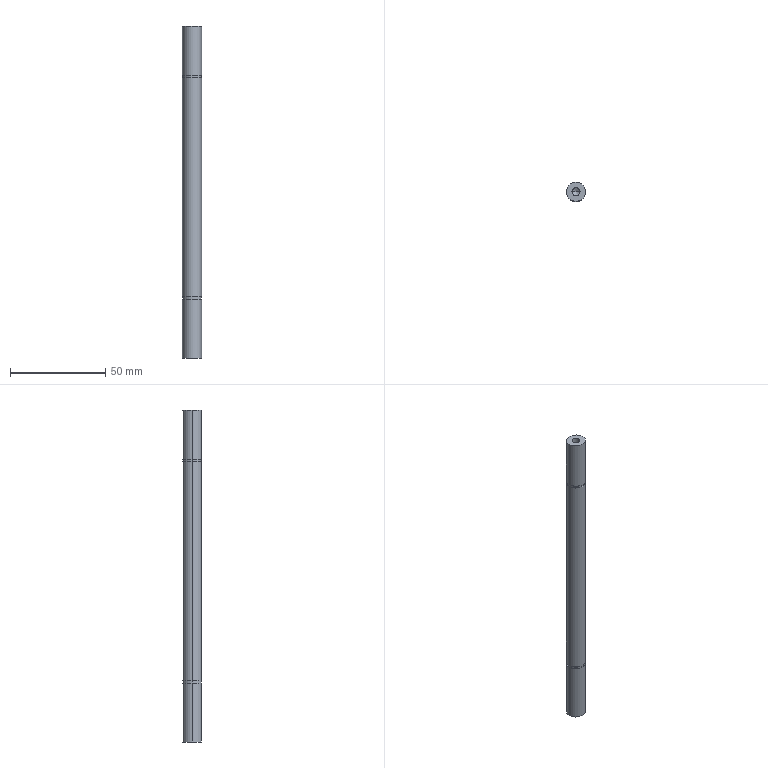Part | SolidWorks | features HoleWzd 2, Extrusion 1, RevCut 1 | 1 solid | 24 faces | box 10 x 10 x 174 mm | volume 13253 mm3 | cylinder 14 | plane 6 | cone 4 | commonest cylinder face diameters 10 x6 4.2 x4 9.6 x4
STEP:
#1=CARTESIAN_POINT('',(5.,0.,-56.1));
#2=VERTEX_POINT('',#1);
#3=CARTESIAN_POINT('',(-5.,0.,-56.1));
#4=VERTEX_POINT('',#3);
#5=CARTESIAN_POINT('',(0.,0.,-56.1));
#6=DIRECTION('',(0.,0.,1.));
#7=DIRECTION('',(1.,0.,0.));
#8=AXIS2_PLACEMENT_3D('',#5,#6,#7);
#9=CIRCLE('',#8,5.);
#10=EDGE_CURVE('',#2,#4,#9,.T.);
#11=ORIENTED_EDGE('',*,*,#10,.F.);
#12=CARTESIAN_POINT('',(5.,0.,-87.));
#13=VERTEX_POINT('',#12);
#14=CARTESIAN_POINT('',(5.,0.,87.));
#15=DIRECTION('',(0.,0.,-1.));
#16=VECTOR('',#15,1000.);
#17=LINE('',#14,#16);
#18=EDGE_CURVE('',#2,#13,#17,.T.);
#19=ORIENTED_EDGE('',*,*,#18,.T.);
#20=CARTESIAN_POINT('',(-5.,0.,-87.));
#21=VERTEX_POINT('',#20);
#22=CARTESIAN_POINT('',(0.,0.,-87.));
#23=DIRECTION('',(0.,0.,1.));
#24=DIRECTION('',(1.,0.,0.));
#25=AXIS2_PLACEMENT_3D('',#22,#23,#24);
#26=CIRCLE('',#25,5.);
#27=EDGE_CURVE('',#13,#21,#26,.T.);
#28=ORIENTED_EDGE('',*,*,#27,.T.);
#29=CARTESIAN_POINT('',(-5.,0.,87.));
#30=DIRECTION('',(0.,0.,-1.));
#31=VECTOR('',#30,1000.);
#32=LINE('',#29,#31);
#33=EDGE_CURVE('',#4,#21,#32,.T.);
#34=ORIENTED_EDGE('',*,*,#33,.F.);
#35=EDGE_LOOP('',(#11,#19,#28,#34));
#36=FACE_OUTER_BOUND('',#35,.T.);
#37=CARTESIAN_POINT('',(0.,0.,87.));
#38=DIRECTION('',(0.,0.,-1.));
#39=DIRECTION('',(-1.,0.,0.));
#40=AXIS2_PLACEMENT_3D('',#37,#38,#39);
#41=CYLINDRICAL_SURFACE('',#40,5.);
#42=ADVANCED_FACE('',(#36),#41,.T.);
#43=CARTESIAN_POINT('',(2.1,0.,-73.));
#44=VERTEX_POINT('',#43);
#45=CARTESIAN_POINT('',(-2.1,0.,-73.));
#46=VERTEX_POINT('',#45);
#47=CARTESIAN_POINT('',(0.,0.,-73.));
#48=DIRECTION('',(0.,0.,-1.));
#49=DIRECTION('',(-1.,0.,0.));
#50=AXIS2_PLACEMENT_3D('',#47,#48,#49);
#51=CIRCLE('',#50,2.1);
#52=EDGE_CURVE('',#44,#46,#51,.T.);
#53=ORIENTED_EDGE('',*,*,#52,.F.);
#54=CARTESIAN_POINT('',(2.1,0.,-87.));
#55=VERTEX_POINT('',#54);
#56=CARTESIAN_POINT('',(2.1,0.,-87.));
#57=DIRECTION('',(0.,0.,-1.));
#58=VECTOR('',#57,1000.);
#59=LINE('',#56,#58);
#60=EDGE_CURVE('',#44,#55,#59,.T.);
#61=ORIENTED_EDGE('',*,*,#60,.T.);
#62=CARTESIAN_POINT('',(-2.1,0.,-87.));
#63=VERTEX_POINT('',#62);
#64=CARTESIAN_POINT('',(0.,0.,-87.));
#65=DIRECTION('',(0.,0.,-1.));
#66=DIRECTION('',(-1.,0.,0.));
#67=AXIS2_PLACEMENT_3D('',#64,#65,#66);
#68=CIRCLE('',#67,2.1);
#69=EDGE_CURVE('',#55,#63,#68,.T.);
#70=ORIENTED_EDGE('',*,*,#69,.T.);
#71=CARTESIAN_POINT('',(-2.1,0.,-87.));
#72=DIRECTION('',(0.,0.,-1.));
#73=VECTOR('',#72,1000.);
#74=LINE('',#71,#73);
#75=EDGE_CURVE('',#46,#63,#74,.T.);
#76=ORIENTED_EDGE('',*,*,#75,.F.);
#77=EDGE_LOOP('',(#53,#61,#70,#76));
#78=FACE_OUTER_BOUND('',#77,.T.);
#79=CARTESIAN_POINT('',(0.,0.,-87.));
#80=DIRECTION('',(0.,0.,-1.));
#81=DIRECTION('',(-1.,0.,0.));
#82=AXIS2_PLACEMENT_3D('',#79,#80,#81);
#83=CYLINDRICAL_SURFACE('',#82,2.1);
#84=ADVANCED_FACE('',(#78),#83,.F.);
#85=CARTESIAN_POINT('',(0.,0.,-71.738));
#86=VERTEX_POINT('',#85);
#87=CARTESIAN_POINT('',(-2.1,0.,-73.));
#88=DIRECTION('',(-0.8572,0.,-0.515));
#89=VECTOR('',#88,1000.);
#90=LINE('',#87,#89);
#91=EDGE_CURVE('',#86,#46,#90,.T.);
#92=ORIENTED_EDGE('',*,*,#91,.F.);
#93=CARTESIAN_POINT('',(2.1,0.,-73.));
#94=DIRECTION('',(0.8572,0.,-0.515));
#95=VECTOR('',#94,1000.);
#96=LINE('',#93,#95);
#97=EDGE_CURVE('',#86,#44,#96,.T.);
#98=ORIENTED_EDGE('',*,*,#97,.T.);
#99=ORIENTED_EDGE('',*,*,#52,.T.);
#100=EDGE_LOOP('',(#92,#98,#99));
#101=FACE_OUTER_BOUND('',#100,.T.);
#102=CARTESIAN_POINT('',(0.,0.,-73.));
#103=DIRECTION('',(0.,0.,-1.));
#104=DIRECTION('',(-1.,0.,0.));
#105=AXIS2_PLACEMENT_3D('',#102,#103,#104);
#106=CONICAL_SURFACE('',#105,2.1,1.03);
#107=ADVANCED_FACE('',(#101),#106,.F.);
#108=CARTESIAN_POINT('',(4.8,0.,-56.1));
#109=VERTEX_POINT('',#108);
#110=CARTESIAN_POINT('',(-4.8,0.,-56.1));
#111=VERTEX_POINT('',#110);
#112=CARTESIAN_POINT('',(0.,0.,-56.1));
#113=DIRECTION('',(0.,0.,1.));
#114=DIRECTION('',(1.,0.,0.));
#115=AXIS2_PLACEMENT_3D('',#112,#113,#114);
#116=CIRCLE('',#115,4.8);
#117=EDGE_CURVE('',#109,#111,#116,.T.);
#118=ORIENTED_EDGE('',*,*,#117,.T.);
#119=CARTESIAN_POINT('',(-4.8,0.,-55.));
#120=VERTEX_POINT('',#119);
#121=CARTESIAN_POINT('',(-4.8,0.,87.));
#122=DIRECTION('',(0.,0.,1.));
#123=VECTOR('',#122,1000.);
#124=LINE('',#121,#123);
#125=EDGE_CURVE('',#111,#120,#124,.T.);
#126=ORIENTED_EDGE('',*,*,#125,.T.);
#127=CARTESIAN_POINT('',(4.8,0.,-55.));
#128=VERTEX_POINT('',#127);
#129=CARTESIAN_POINT('',(0.,0.,-55.));
#130=DIRECTION('',(0.,0.,1.));
#131=DIRECTION('',(1.,0.,0.));
#132=AXIS2_PLACEMENT_3D('',#129,#130,#131);
#133=CIRCLE('',#132,4.8);
#134=EDGE_CURVE('',#128,#120,#133,.T.);
#135=ORIENTED_EDGE('',*,*,#134,.F.);
#136=CARTESIAN_POINT('',(4.8,0.,87.));
#137=DIRECTION('',(0.,0.,1.));
#138=VECTOR('',#137,1000.);
#139=LINE('',#136,#138);
#140=EDGE_CURVE('',#109,#128,#139,.T.);
#141=ORIENTED_EDGE('',*,*,#140,.F.);
#142=EDGE_LOOP('',(#118,#126,#135,#141));
#143=FACE_OUTER_BOUND('',#142,.T.);
#144=CARTESIAN_POINT('',(0.,0.,87.));
#145=DIRECTION('',(0.,0.,1.));
#146=DIRECTION('',(1.,0.,0.));
#147=AXIS2_PLACEMENT_3D('',#144,#145,#146);
#148=CYLINDRICAL_SURFACE('',#147,4.8);
#149=ADVANCED_FACE('',(#143),#148,.T.);
#150=CARTESIAN_POINT('',(4.8,0.,60.));
#151=VERTEX_POINT('',#150);
#152=CARTESIAN_POINT('',(-4.8,0.,60.));
#153=VERTEX_POINT('',#152);
#154=CARTESIAN_POINT('',(0.,0.,60.));
#155=DIRECTION('',(0.,0.,1.));
#156=DIRECTION('',(1.,0.,0.));
#157=AXIS2_PLACEMENT_3D('',#154,#155,#156);
#158=CIRCLE('',#157,4.8);
#159=EDGE_CURVE('',#151,#153,#158,.T.);
#160=ORIENTED_EDGE('',*,*,#159,.T.);
#161=CARTESIAN_POINT('',(-4.8,0.,61.1));
#162=VERTEX_POINT('',#161);
#163=CARTESIAN_POINT('',(-4.8,0.,87.));
#164=DIRECTION('',(0.,0.,1.));
#165=VECTOR('',#164,1000.);
#166=LINE('',#163,#165);
#167=EDGE_CURVE('',#153,#162,#166,.T.);
#168=ORIENTED_EDGE('',*,*,#167,.T.);
#169=CARTESIAN_POINT('',(4.8,0.,61.1));
#170=VERTEX_POINT('',#169);
#171=CARTESIAN_POINT('',(0.,0.,61.1));
#172=DIRECTION('',(0.,0.,1.));
#173=DIRECTION('',(1.,0.,0.));
#174=AXIS2_PLACEMENT_3D('',#171,#172,#173);
#175=CIRCLE('',#174,4.8);
#176=EDGE_CURVE('',#170,#162,#175,.T.);
#177=ORIENTED_EDGE('',*,*,#176,.F.);
#178=CARTESIAN_POINT('',(4.8,0.,87.));
#179=DIRECTION('',(0.,0.,1.));
#180=VECTOR('',#179,1000.);
#181=LINE('',#178,#180);
#182=EDGE_CURVE('',#151,#170,#181,.T.);
#183=ORIENTED_EDGE('',*,*,#182,.F.);
#184=EDGE_LOOP('',(#160,#168,#177,#183));
#185=FACE_OUTER_BOUND('',#184,.T.);
#186=CARTESIAN_POINT('',(0.,0.,87.));
#187=DIRECTION('',(0.,0.,1.));
#188=DIRECTION('',(1.,0.,0.));
#189=AXIS2_PLACEMENT_3D('',#186,#187,#188);
#190=CYLINDRICAL_SURFACE('',#189,4.8);
#191=ADVANCED_FACE('',(#185),#190,.T.);
#192=CARTESIAN_POINT('',(-2.1,0.,73.));
#193=VERTEX_POINT('',#192);
#194=CARTESIAN_POINT('',(2.1,0.,73.));
#195=VERTEX_POINT('',#194);
#196=CARTESIAN_POINT('',(0.,0.,73.));
#197=DIRECTION('',(0.,0.,1.));
#198=DIRECTION('',(1.,0.,0.));
#199=AXIS2_PLACEMENT_3D('',#196,#197,#198);
#200=CIRCLE('',#199,2.1);
#201=EDGE_CURVE('',#193,#195,#200,.T.);
#202=ORIENTED_EDGE('',*,*,#201,.F.);
#203=CARTESIAN_POINT('',(-2.1,0.,87.));
#204=VERTEX_POINT('',#203);
#205=CARTESIAN_POINT('',(-2.1,0.,87.));
#206=DIRECTION('',(0.,0.,1.));
#207=VECTOR('',#206,1000.);
#208=LINE('',#205,#207);
#209=EDGE_CURVE('',#193,#204,#208,.T.);
#210=ORIENTED_EDGE('',*,*,#209,.T.);
#211=CARTESIAN_POINT('',(2.1,0.,87.));
#212=VERTEX_POINT('',#211);
#213=CARTESIAN_POINT('',(0.,0.,87.));
#214=DIRECTION('',(0.,0.,1.));
#215=DIRECTION('',(1.,0.,0.));
#216=AXIS2_PLACEMENT_3D('',#213,#214,#215);
#217=CIRCLE('',#216,2.1);
#218=EDGE_CURVE('',#204,#212,#217,.T.);
#219=ORIENTED_EDGE('',*,*,#218,.T.);
#220=CARTESIAN_POINT('',(2.1,0.,87.));
#221=DIRECTION('',(0.,0.,1.));
#222=VECTOR('',#221,1000.);
#223=LINE('',#220,#222);
#224=EDGE_CURVE('',#195,#212,#223,.T.);
#225=ORIENTED_EDGE('',*,*,#224,.F.);
#226=EDGE_LOOP('',(#202,#210,#219,#225));
#227=FACE_OUTER_BOUND('',#226,.T.);
#228=CARTESIAN_POINT('',(0.,0.,87.));
#229=DIRECTION('',(0.,0.,1.));
#230=DIRECTION('',(1.,0.,0.));
#231=AXIS2_PLACEMENT_3D('',#228,#229,#230);
#232=CYLINDRICAL_SURFACE('',#231,2.1);
#233=ADVANCED_FACE('',(#227),#232,.F.);
#234=CARTESIAN_POINT('',(0.,0.,71.738));
#235=VERTEX_POINT('',#234);
#236=CARTESIAN_POINT('',(2.1,0.,73.));
#237=DIRECTION('',(0.8572,0.,0.515));
#238=VECTOR('',#237,1000.);
#239=LINE('',#236,#238);
#240=EDGE_CURVE('',#235,#195,#239,.T.);
#241=ORIENTED_EDGE('',*,*,#240,.F.);
#242=CARTESIAN_POINT('',(-2.1,0.,73.));
#243=DIRECTION('',(-0.8572,0.,0.515));
#244=VECTOR('',#243,1000.);
#245=LINE('',#242,#244);
#246=EDGE_CURVE('',#235,#193,#245,.T.);
#247=ORIENTED_EDGE('',*,*,#246,.T.);
#248=ORIENTED_EDGE('',*,*,#201,.T.);
#249=EDGE_LOOP('',(#241,#247,#248));
#250=FACE_OUTER_BOUND('',#249,.T.);
#251=CARTESIAN_POINT('',(0.,0.,73.));
#252=DIRECTION('',(0.,0.,1.));
#253=DIRECTION('',(1.,0.,0.));
#254=AXIS2_PLACEMENT_3D('',#251,#252,#253);
#255=CONICAL_SURFACE('',#254,2.1,1.03);
#256=ADVANCED_FACE('',(#250),#255,.F.);
#257=CARTESIAN_POINT('',(5.,0.,87.));
#258=VERTEX_POINT('',#257);
#259=CARTESIAN_POINT('',(-5.,0.,87.));
#260=VERTEX_POINT('',#259);
#261=CARTESIAN_POINT('',(0.,0.,87.));
#262=DIRECTION('',(0.,0.,1.));
#263=DIRECTION('',(1.,0.,0.));
#264=AXIS2_PLACEMENT_3D('',#261,#262,#263);
#265=CIRCLE('',#264,5.);
#266=EDGE_CURVE('',#258,#260,#265,.T.);
#267=ORIENTED_EDGE('',*,*,#266,.F.);
#268=CARTESIAN_POINT('',(5.,0.,61.1));
#269=VERTEX_POINT('',#268);
#270=CARTESIAN_POINT('',(5.,0.,87.));
#271=DIRECTION('',(0.,0.,-1.));
#272=VECTOR('',#271,1000.);
#273=LINE('',#270,#272);
#274=EDGE_CURVE('',#258,#269,#273,.T.);
#275=ORIENTED_EDGE('',*,*,#274,.T.);
#276=CARTESIAN_POINT('',(-5.,0.,61.1));
#277=VERTEX_POINT('',#276);
#278=CARTESIAN_POINT('',(0.,0.,61.1));
#279=DIRECTION('',(0.,0.,1.));
#280=DIRECTION('',(1.,0.,0.));
#281=AXIS2_PLACEMENT_3D('',#278,#279,#280);
#282=CIRCLE('',#281,5.);
#283=EDGE_CURVE('',#269,#277,#282,.T.);
#284=ORIENTED_EDGE('',*,*,#283,.T.);
#285=CARTESIAN_POINT('',(-5.,0.,87.));
#286=DIRECTION('',(0.,0.,-1.));
#287=VECTOR('',#286,1000.);
#288=LINE('',#285,#287);
#289=EDGE_CURVE('',#260,#277,#288,.T.);
#290=ORIENTED_EDGE('',*,*,#289,.F.);
#291=EDGE_LOOP('',(#267,#275,#284,#290));
#292=FACE_OUTER_BOUND('',#291,.T.);
#293=CARTESIAN_POINT('',(0.,0.,87.));
#294=DIRECTION('',(0.,0.,-1.));
#295=DIRECTION('',(-1.,0.,0.));
#296=AXIS2_PLACEMENT_3D('',#293,#294,#295);
#297=CYLINDRICAL_SURFACE('',#296,5.);
#298=ADVANCED_FACE('',(#292),#297,.T.);
#299=CARTESIAN_POINT('',(5.,0.,60.));
#300=VERTEX_POINT('',#299);
#301=CARTESIAN_POINT('',(-5.,0.,60.));
#302=VERTEX_POINT('',#301);
#303=CARTESIAN_POINT('',(0.,0.,60.));
#304=DIRECTION('',(0.,0.,1.));
#305=DIRECTION('',(1.,0.,0.));
#306=AXIS2_PLACEMENT_3D('',#303,#304,#305);
#307=CIRCLE('',#306,5.);
#308=EDGE_CURVE('',#300,#302,#307,.T.);
#309=ORIENTED_EDGE('',*,*,#308,.F.);
#310=CARTESIAN_POINT('',(5.,0.,-55.));
#311=VERTEX_POINT('',#310);
#312=CARTESIAN_POINT('',(5.,0.,87.));
#313=DIRECTION('',(0.,0.,-1.));
#314=VECTOR('',#313,1000.);
#315=LINE('',#312,#314);
#316=EDGE_CURVE('',#300,#311,#315,.T.);
#317=ORIENTED_EDGE('',*,*,#316,.T.);
#318=CARTESIAN_POINT('',(-5.,0.,-55.));
#319=VERTEX_POINT('',#318);
#320=CARTESIAN_POINT('',(0.,0.,-55.));
#321=DIRECTION('',(0.,0.,1.));
#322=DIRECTION('',(1.,0.,0.));
#323=AXIS2_PLACEMENT_3D('',#320,#321,#322);
#324=CIRCLE('',#323,5.);
#325=EDGE_CURVE('',#311,#319,#324,.T.);
#326=ORIENTED_EDGE('',*,*,#325,.T.);
#327=CARTESIAN_POINT('',(-5.,0.,87.));
#328=DIRECTION('',(0.,0.,-1.));
#329=VECTOR('',#328,1000.);
#330=LINE('',#327,#329);
#331=EDGE_CURVE('',#302,#319,#330,.T.);
#332=ORIENTED_EDGE('',*,*,#331,.F.);
#333=EDGE_LOOP('',(#309,#317,#326,#332));
#334=FACE_OUTER_BOUND('',#333,.T.);
#335=CARTESIAN_POINT('',(0.,0.,87.));
#336=DIRECTION('',(0.,0.,-1.));
#337=DIRECTION('',(-1.,0.,0.));
#338=AXIS2_PLACEMENT_3D('',#335,#336,#337);
#339=CYLINDRICAL_SURFACE('',#338,5.);
#340=ADVANCED_FACE('',(#334),#339,.T.);
#341=ORIENTED_EDGE('',*,*,#316,.F.);
#342=CARTESIAN_POINT('',(0.,0.,60.));
#343=DIRECTION('',(0.,0.,1.));
#344=DIRECTION('',(1.,0.,0.));
#345=AXIS2_PLACEMENT_3D('',#342,#343,#344);
#346=CIRCLE('',#345,5.);
#347=EDGE_CURVE('',#302,#300,#346,.T.);
#348=ORIENTED_EDGE('',*,*,#347,.F.);
#349=ORIENTED_EDGE('',*,*,#331,.T.);
#350=CARTESIAN_POINT('',(0.,0.,-55.));
#351=DIRECTION('',(0.,0.,1.));
#352=DIRECTION('',(1.,0.,0.));
#353=AXIS2_PLACEMENT_3D('',#350,#351,#352);
#354=CIRCLE('',#353,5.);
#355=EDGE_CURVE('',#319,#311,#354,.T.);
#356=ORIENTED_EDGE('',*,*,#355,.T.);
#357=EDGE_LOOP('',(#341,#348,#349,#356));
#358=FACE_OUTER_BOUND('',#357,.T.);
#359=CARTESIAN_POINT('',(0.,0.,87.));
#360=DIRECTION('',(0.,0.,-1.));
#361=DIRECTION('',(-1.,0.,0.));
#362=AXIS2_PLACEMENT_3D('',#359,#360,#361);
#363=CYLINDRICAL_SURFACE('',#362,5.);
#364=ADVANCED_FACE('',(#358),#363,.T.);
#365=ORIENTED_EDGE('',*,*,#274,.F.);
#366=CARTESIAN_POINT('',(0.,0.,87.));
#367=DIRECTION('',(0.,0.,1.));
#368=DIRECTION('',(1.,0.,0.));
#369=AXIS2_PLACEMENT_3D('',#366,#367,#368);
#370=CIRCLE('',#369,5.);
#371=EDGE_CURVE('',#260,#258,#370,.T.);
#372=ORIENTED_EDGE('',*,*,#371,.F.);
#373=ORIENTED_EDGE('',*,*,#289,.T.);
#374=CARTESIAN_POINT('',(0.,0.,61.1));
#375=DIRECTION('',(0.,0.,1.));
#376=DIRECTION('',(1.,0.,0.));
#377=AXIS2_PLACEMENT_3D('',#374,#375,#376);
#378=CIRCLE('',#377,5.);
#379=EDGE_CURVE('',#277,#269,#378,.T.);
#380=ORIENTED_EDGE('',*,*,#379,.T.);
#381=EDGE_LOOP('',(#365,#372,#373,#380));
#382=FACE_OUTER_BOUND('',#381,.T.);
#383=CARTESIAN_POINT('',(0.,0.,87.));
#384=DIRECTION('',(0.,0.,-1.));
#385=DIRECTION('',(-1.,0.,0.));
#386=AXIS2_PLACEMENT_3D('',#383,#384,#385);
#387=CYLINDRICAL_SURFACE('',#386,5.);
#388=ADVANCED_FACE('',(#382),#387,.T.);
#389=CARTESIAN_POINT('',(0.,0.,87.));
#390=DIRECTION('',(0.,0.,1.));
#391=DIRECTION('',(1.,0.,0.));
#392=AXIS2_PLACEMENT_3D('',#389,#390,#391);
#393=CIRCLE('',#392,2.1);
#394=EDGE_CURVE('',#212,#204,#393,.T.);
#395=ORIENTED_EDGE('',*,*,#394,.F.);
#396=ORIENTED_EDGE('',*,*,#218,.F.);
#397=EDGE_LOOP('',(#395,#396));
#398=FACE_BOUND('',#397,.T.);
#399=ORIENTED_EDGE('',*,*,#371,.T.);
#400=ORIENTED_EDGE('',*,*,#266,.T.);
#401=EDGE_LOOP('',(#399,#400));
#402=FACE_OUTER_BOUND('',#401,.T.);
#403=CARTESIAN_POINT('',(0.,0.,87.));
#404=DIRECTION('',(0.,0.,1.));
#405=DIRECTION('',(1.,0.,0.));
#406=AXIS2_PLACEMENT_3D('',#403,#404,#405);
#407=PLANE('',#406);
#408=ADVANCED_FACE('',(#398,#402),#407,.T.);
#409=ORIENTED_EDGE('',*,*,#246,.F.);
#410=ORIENTED_EDGE('',*,*,#240,.T.);
#411=CARTESIAN_POINT('',(0.,0.,73.));
#412=DIRECTION('',(0.,0.,1.));
#413=DIRECTION('',(1.,0.,0.));
#414=AXIS2_PLACEMENT_3D('',#411,#412,#413);
#415=CIRCLE('',#414,2.1);
#416=EDGE_CURVE('',#195,#193,#415,.T.);
#417=ORIENTED_EDGE('',*,*,#416,.T.);
#418=EDGE_LOOP('',(#409,#410,#417));
#419=FACE_OUTER_BOUND('',#418,.T.);
#420=CARTESIAN_POINT('',(0.,0.,73.));
#421=DIRECTION('',(0.,0.,1.));
#422=DIRECTION('',(1.,0.,0.));
#423=AXIS2_PLACEMENT_3D('',#420,#421,#422);
#424=CONICAL_SURFACE('',#423,2.1,1.03);
#425=ADVANCED_FACE('',(#419),#424,.F.);
#426=ORIENTED_EDGE('',*,*,#209,.F.);
#427=ORIENTED_EDGE('',*,*,#416,.F.);
#428=ORIENTED_EDGE('',*,*,#224,.T.);
#429=ORIENTED_EDGE('',*,*,#394,.T.);
#430=EDGE_LOOP('',(#426,#427,#428,#429));
#431=FACE_OUTER_BOUND('',#430,.T.);
#432=CARTESIAN_POINT('',(0.,0.,87.));
#433=DIRECTION('',(0.,0.,1.));
#434=DIRECTION('',(1.,0.,0.));
#435=AXIS2_PLACEMENT_3D('',#432,#433,#434);
#436=CYLINDRICAL_SURFACE('',#435,2.1);
#437=ADVANCED_FACE('',(#431),#436,.F.);
#438=ORIENTED_EDGE('',*,*,#176,.T.);
#439=CARTESIAN_POINT('',(0.,0.,61.1));
#440=DIRECTION('',(0.,0.,1.));
#441=DIRECTION('',(1.,0.,0.));
#442=AXIS2_PLACEMENT_3D('',#439,#440,#441);
#443=CIRCLE('',#442,4.8);
#444=EDGE_CURVE('',#162,#170,#443,.T.);
#445=ORIENTED_EDGE('',*,*,#444,.T.);
#446=EDGE_LOOP('',(#438,#445));
#447=FACE_BOUND('',#446,.T.);
#448=ORIENTED_EDGE('',*,*,#379,.F.);
#449=ORIENTED_EDGE('',*,*,#283,.F.);
#450=EDGE_LOOP('',(#448,#449));
#451=FACE_OUTER_BOUND('',#450,.T.);
#452=CARTESIAN_POINT('',(0.,5.,61.1));
#453=DIRECTION('',(0.,0.,-1.));
#454=DIRECTION('',(-1.,0.,0.));
#455=AXIS2_PLACEMENT_3D('',#452,#453,#454);
#456=PLANE('',#455);
#457=ADVANCED_FACE('',(#447,#451),#456,.T.);
#458=ORIENTED_EDGE('',*,*,#167,.F.);
#459=CARTESIAN_POINT('',(0.,0.,60.));
#460=DIRECTION('',(0.,0.,1.));
#461=DIRECTION('',(1.,0.,0.));
#462=AXIS2_PLACEMENT_3D('',#459,#460,#461);
#463=CIRCLE('',#462,4.8);
#464=EDGE_CURVE('',#153,#151,#463,.T.);
#465=ORIENTED_EDGE('',*,*,#464,.T.);
#466=ORIENTED_EDGE('',*,*,#182,.T.);
#467=ORIENTED_EDGE('',*,*,#444,.F.);
#468=EDGE_LOOP('',(#458,#465,#466,#467));
#469=FACE_OUTER_BOUND('',#468,.T.);
#470=CARTESIAN_POINT('',(0.,0.,87.));
#471=DIRECTION('',(0.,0.,1.));
#472=DIRECTION('',(1.,0.,0.));
#473=AXIS2_PLACEMENT_3D('',#470,#471,#472);
#474=CYLINDRICAL_SURFACE('',#473,4.8);
#475=ADVANCED_FACE('',(#469),#474,.T.);
#476=ORIENTED_EDGE('',*,*,#347,.T.);
#477=ORIENTED_EDGE('',*,*,#308,.T.);
#478=EDGE_LOOP('',(#476,#477));
#479=FACE_OUTER_BOUND('',#478,.T.);
#480=ORIENTED_EDGE('',*,*,#159,.F.);
#481=ORIENTED_EDGE('',*,*,#464,.F.);
#482=EDGE_LOOP('',(#480,#481));
#483=FACE_BOUND('',#482,.T.);
#484=CARTESIAN_POINT('',(0.,5.,60.));
#485=DIRECTION('',(0.,0.,1.));
#486=DIRECTION('',(1.,0.,0.));
#487=AXIS2_PLACEMENT_3D('',#484,#485,#486);
#488=PLANE('',#487);
#489=ADVANCED_FACE('',(#479,#483),#488,.T.);
#490=ORIENTED_EDGE('',*,*,#134,.T.);
#491=CARTESIAN_POINT('',(0.,0.,-55.));
#492=DIRECTION('',(0.,0.,1.));
#493=DIRECTION('',(1.,0.,0.));
#494=AXIS2_PLACEMENT_3D('',#491,#492,#493);
#495=CIRCLE('',#494,4.8);
#496=EDGE_CURVE('',#120,#128,#495,.T.);
#497=ORIENTED_EDGE('',*,*,#496,.T.);
#498=EDGE_LOOP('',(#490,#497));
#499=FACE_BOUND('',#498,.T.);
#500=ORIENTED_EDGE('',*,*,#355,.F.);
#501=ORIENTED_EDGE('',*,*,#325,.F.);
#502=EDGE_LOOP('',(#500,#501));
#503=FACE_OUTER_BOUND('',#502,.T.);
#504=CARTESIAN_POINT('',(0.,5.,-55.));
#505=DIRECTION('',(0.,0.,-1.));
#506=DIRECTION('',(-1.,0.,0.));
#507=AXIS2_PLACEMENT_3D('',#504,#505,#506);
#508=PLANE('',#507);
#509=ADVANCED_FACE('',(#499,#503),#508,.T.);
#510=ORIENTED_EDGE('',*,*,#125,.F.);
#511=CARTESIAN_POINT('',(0.,0.,-56.1));
#512=DIRECTION('',(0.,0.,1.));
#513=DIRECTION('',(1.,0.,0.));
#514=AXIS2_PLACEMENT_3D('',#511,#512,#513);
#515=CIRCLE('',#514,4.8);
#516=EDGE_CURVE('',#111,#109,#515,.T.);
#517=ORIENTED_EDGE('',*,*,#516,.T.);
#518=ORIENTED_EDGE('',*,*,#140,.T.);
#519=ORIENTED_EDGE('',*,*,#496,.F.);
#520=EDGE_LOOP('',(#510,#517,#518,#519));
#521=FACE_OUTER_BOUND('',#520,.T.);
#522=CARTESIAN_POINT('',(0.,0.,87.));
#523=DIRECTION('',(0.,0.,1.));
#524=DIRECTION('',(1.,0.,0.));
#525=AXIS2_PLACEMENT_3D('',#522,#523,#524);
#526=CYLINDRICAL_SURFACE('',#525,4.8);
#527=ADVANCED_FACE('',(#521),#526,.T.);
#528=CARTESIAN_POINT('',(0.,0.,-56.1));
#529=DIRECTION('',(0.,0.,1.));
#530=DIRECTION('',(1.,0.,0.));
#531=AXIS2_PLACEMENT_3D('',#528,#529,#530);
#532=CIRCLE('',#531,5.);
#533=EDGE_CURVE('',#4,#2,#532,.T.);
#534=ORIENTED_EDGE('',*,*,#533,.T.);
#535=ORIENTED_EDGE('',*,*,#10,.T.);
#536=EDGE_LOOP('',(#534,#535));
#537=FACE_OUTER_BOUND('',#536,.T.);
#538=ORIENTED_EDGE('',*,*,#117,.F.);
#539=ORIENTED_EDGE('',*,*,#516,.F.);
#540=EDGE_LOOP('',(#538,#539));
#541=FACE_BOUND('',#540,.T.);
#542=CARTESIAN_POINT('',(0.,5.,-56.1));
#543=DIRECTION('',(0.,0.,1.));
#544=DIRECTION('',(1.,0.,0.));
#545=AXIS2_PLACEMENT_3D('',#542,#543,#544);
#546=PLANE('',#545);
#547=ADVANCED_FACE('',(#537,#541),#546,.T.);
#548=ORIENTED_EDGE('',*,*,#97,.F.);
#549=ORIENTED_EDGE('',*,*,#91,.T.);
#550=CARTESIAN_POINT('',(0.,0.,-73.));
#551=DIRECTION('',(0.,0.,-1.));
#552=DIRECTION('',(-1.,0.,0.));
#553=AXIS2_PLACEMENT_3D('',#550,#551,#552);
#554=CIRCLE('',#553,2.1);
#555=EDGE_CURVE('',#46,#44,#554,.T.);
#556=ORIENTED_EDGE('',*,*,#555,.T.);
#557=EDGE_LOOP('',(#548,#549,#556));
#558=FACE_OUTER_BOUND('',#557,.T.);
#559=CARTESIAN_POINT('',(0.,0.,-73.));
#560=DIRECTION('',(0.,0.,-1.));
#561=DIRECTION('',(-1.,0.,0.));
#562=AXIS2_PLACEMENT_3D('',#559,#560,#561);
#563=CONICAL_SURFACE('',#562,2.1,1.03);
#564=ADVANCED_FACE('',(#558),#563,.F.);
#565=ORIENTED_EDGE('',*,*,#60,.F.);
#566=ORIENTED_EDGE('',*,*,#555,.F.);
#567=ORIENTED_EDGE('',*,*,#75,.T.);
#568=CARTESIAN_POINT('',(0.,0.,-87.));
#569=DIRECTION('',(0.,0.,-1.));
#570=DIRECTION('',(-1.,0.,0.));
#571=AXIS2_PLACEMENT_3D('',#568,#569,#570);
#572=CIRCLE('',#571,2.1);
#573=EDGE_CURVE('',#63,#55,#572,.T.);
#574=ORIENTED_EDGE('',*,*,#573,.T.);
#575=EDGE_LOOP('',(#565,#566,#567,#574));
#576=FACE_OUTER_BOUND('',#575,.T.);
#577=CARTESIAN_POINT('',(0.,0.,-87.));
#578=DIRECTION('',(0.,0.,-1.));
#579=DIRECTION('',(-1.,0.,0.));
#580=AXIS2_PLACEMENT_3D('',#577,#578,#579);
#581=CYLINDRICAL_SURFACE('',#580,2.1);
#582=ADVANCED_FACE('',(#576),#581,.F.);
#583=ORIENTED_EDGE('',*,*,#573,.F.);
#584=ORIENTED_EDGE('',*,*,#69,.F.);
#585=EDGE_LOOP('',(#583,#584));
#586=FACE_BOUND('',#585,.T.);
#587=CARTESIAN_POINT('',(0.,0.,-87.));
#588=DIRECTION('',(0.,0.,1.));
#589=DIRECTION('',(1.,0.,0.));
#590=AXIS2_PLACEMENT_3D('',#587,#588,#589);
#591=CIRCLE('',#590,5.);
#592=EDGE_CURVE('',#21,#13,#591,.T.);
#593=ORIENTED_EDGE('',*,*,#592,.F.);
#594=ORIENTED_EDGE('',*,*,#27,.F.);
#595=EDGE_LOOP('',(#593,#594));
#596=FACE_OUTER_BOUND('',#595,.T.);
#597=CARTESIAN_POINT('',(0.,0.,-87.));
#598=DIRECTION('',(0.,0.,1.));
#599=DIRECTION('',(1.,0.,0.));
#600=AXIS2_PLACEMENT_3D('',#597,#598,#599);
#601=PLANE('',#600);
#602=ADVANCED_FACE('',(#586,#596),#601,.F.);
#603=ORIENTED_EDGE('',*,*,#18,.F.);
#604=ORIENTED_EDGE('',*,*,#533,.F.);
#605=ORIENTED_EDGE('',*,*,#33,.T.);
#606=ORIENTED_EDGE('',*,*,#592,.T.);
#607=EDGE_LOOP('',(#603,#604,#605,#606));
#608=FACE_OUTER_BOUND('',#607,.T.);
#609=CARTESIAN_POINT('',(0.,0.,87.));
#610=DIRECTION('',(0.,0.,-1.));
#611=DIRECTION('',(-1.,0.,0.));
#612=AXIS2_PLACEMENT_3D('',#609,#610,#611);
#613=CYLINDRICAL_SURFACE('',#612,5.);
#614=ADVANCED_FACE('',(#608),#613,.T.);
#615=CLOSED_SHELL('',(#42,#84,#107,#149,#191,#233,#256,#298,#340,#364,#388,#408,#425,#437,#457,#475,#489,#509,#527,#547,#564,#582,#602,#614));
#616=MANIFOLD_SOLID_BREP('',#615);
#617=CARTESIAN_POINT('',(0.,0.,0.));
#618=DIRECTION('',(0.,0.,1.));
#619=DIRECTION('',(1.,0.,0.));
#620=AXIS2_PLACEMENT_3D('',#617,#618,#619);
#621=(LENGTH_UNIT()NAMED_UNIT(*)SI_UNIT(.MILLI.,.METRE.));
#622=UNCERTAINTY_MEASURE_WITH_UNIT(LENGTH_MEASURE(0.00001),#621,'','');
#623=(NAMED_UNIT(*)PLANE_ANGLE_UNIT()SI_UNIT($,.RADIAN.));
#624=(NAMED_UNIT(*)SI_UNIT($,.STERADIAN.)SOLID_ANGLE_UNIT());
#625=(GEOMETRIC_REPRESENTATION_CONTEXT(3)GLOBAL_UNCERTAINTY_ASSIGNED_CONTEXT((#622))GLOBAL_UNIT_ASSIGNED_CONTEXT((#621,#623,#624))REPRESENTATION_CONTEXT('',''));
#626=ADVANCED_BREP_SHAPE_REPRESENTATION('',(#616,#620),#625);